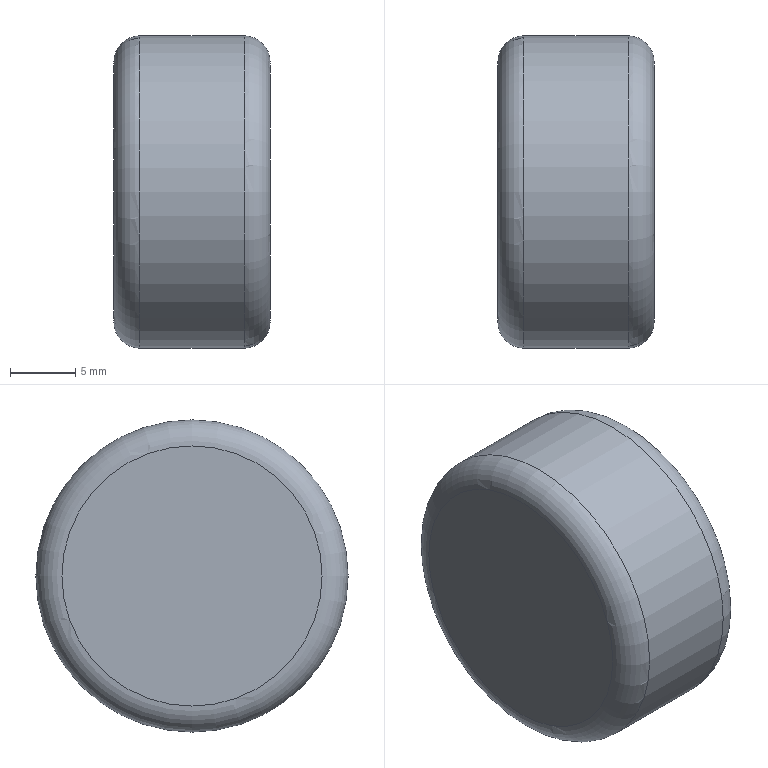Part | NX | features solid 2 | 1 solid | 5 faces | box 12 x 24 x 24 mm | volume 5304 mm3 | plane 2 | torus 2 | cylinder 1 | commonest cylinder face diameters 24 x1
STEP:
#1=CARTESIAN_POINT('',(-73.,145.3,106.));
#2=VERTEX_POINT('',#1);
#3=CARTESIAN_POINT('',(-73.,145.3,96.));
#4=DIRECTION('',(-1.,0.,0.));
#5=DIRECTION('',(0.,0.,1.));
#6=AXIS2_PLACEMENT_3D('',#3,#4,#5);
#7=CIRCLE('',#6,10.);
#8=EDGE_CURVE('',#2,#2,#7,.T.);
#9=ORIENTED_EDGE('',*,*,#8,.T.);
#10=EDGE_LOOP('',(#9));
#11=FACE_BOUND('',#10,.T.);
#12=CARTESIAN_POINT('',(-73.,145.3,96.));
#13=DIRECTION('',(-1.,0.,0.));
#14=DIRECTION('',(0.,0.,1.));
#15=AXIS2_PLACEMENT_3D('',#12,#13,#14);
#16=PLANE('',#15);
#17=ADVANCED_FACE('',(#11),#16,.T.);
#18=CARTESIAN_POINT('',(-61.,145.3,86.));
#19=VERTEX_POINT('',#18);
#20=CARTESIAN_POINT('',(-61.,145.3,96.));
#21=DIRECTION('',(1.,0.,0.));
#22=DIRECTION('',(0.,0.,-1.));
#23=AXIS2_PLACEMENT_3D('',#20,#21,#22);
#24=CIRCLE('',#23,10.);
#25=EDGE_CURVE('',#19,#19,#24,.T.);
#26=ORIENTED_EDGE('',*,*,#25,.T.);
#27=EDGE_LOOP('',(#26));
#28=FACE_BOUND('',#27,.T.);
#29=CARTESIAN_POINT('',(-61.,145.3,96.));
#30=DIRECTION('',(1.,0.,0.));
#31=DIRECTION('',(0.,0.,-1.));
#32=AXIS2_PLACEMENT_3D('',#29,#30,#31);
#33=PLANE('',#32);
#34=ADVANCED_FACE('',(#28),#33,.T.);
#35=CARTESIAN_POINT('',(-71.,145.3,108.));
#36=VERTEX_POINT('',#35);
#37=CARTESIAN_POINT('',(-71.,145.3,96.));
#38=DIRECTION('',(-1.,0.,0.));
#39=DIRECTION('',(0.,0.,1.));
#40=AXIS2_PLACEMENT_3D('',#37,#38,#39);
#41=CIRCLE('',#40,12.);
#42=EDGE_CURVE('',#36,#36,#41,.F.);
#43=ORIENTED_EDGE('',*,*,#42,.T.);
#44=EDGE_LOOP('',(#43));
#45=FACE_BOUND('',#44,.T.);
#46=CARTESIAN_POINT('',(-63.,145.3,84.));
#47=VERTEX_POINT('',#46);
#48=CARTESIAN_POINT('',(-63.,145.3,96.));
#49=DIRECTION('',(1.,0.,0.));
#50=DIRECTION('',(0.,0.,-1.));
#51=AXIS2_PLACEMENT_3D('',#48,#49,#50);
#52=CIRCLE('',#51,12.);
#53=EDGE_CURVE('',#47,#47,#52,.F.);
#54=ORIENTED_EDGE('',*,*,#53,.T.);
#55=EDGE_LOOP('',(#54));
#56=FACE_BOUND('',#55,.T.);
#57=CARTESIAN_POINT('',(-61.,145.3,96.));
#58=DIRECTION('',(-1.,0.,0.));
#59=DIRECTION('',(0.,0.,1.));
#60=AXIS2_PLACEMENT_3D('',#57,#58,#59);
#61=CYLINDRICAL_SURFACE('',#60,12.);
#62=ADVANCED_FACE('',(#45,#56),#61,.T.);
#63=ORIENTED_EDGE('',*,*,#8,.F.);
#64=EDGE_LOOP('',(#63));
#65=FACE_BOUND('',#64,.T.);
#66=ORIENTED_EDGE('',*,*,#42,.F.);
#67=EDGE_LOOP('',(#66));
#68=FACE_BOUND('',#67,.T.);
#69=CARTESIAN_POINT('',(-71.,145.3,96.));
#70=DIRECTION('',(-1.,0.,0.));
#71=DIRECTION('',(0.,0.,1.));
#72=AXIS2_PLACEMENT_3D('',#69,#70,#71);
#73=TOROIDAL_SURFACE('',#72,10.,2.);
#74=ADVANCED_FACE('',(#65,#68),#73,.T.);
#75=ORIENTED_EDGE('',*,*,#25,.F.);
#76=EDGE_LOOP('',(#75));
#77=FACE_BOUND('',#76,.T.);
#78=ORIENTED_EDGE('',*,*,#53,.F.);
#79=EDGE_LOOP('',(#78));
#80=FACE_BOUND('',#79,.T.);
#81=CARTESIAN_POINT('',(-63.,145.3,96.));
#82=DIRECTION('',(1.,0.,0.));
#83=DIRECTION('',(0.,0.,-1.));
#84=AXIS2_PLACEMENT_3D('',#81,#82,#83);
#85=TOROIDAL_SURFACE('',#84,10.,2.);
#86=ADVANCED_FACE('',(#77,#80),#85,.T.);
#87=CLOSED_SHELL('',(#17,#34,#62,#74,#86));
#88=MANIFOLD_SOLID_BREP('',#87);
#89=(LENGTH_UNIT()NAMED_UNIT(*)SI_UNIT(.MILLI.,.METRE.));
#90=UNCERTAINTY_MEASURE_WITH_UNIT(LENGTH_MEASURE(0.00001),#89,'','');
#91=(NAMED_UNIT(*)PLANE_ANGLE_UNIT()SI_UNIT($,.RADIAN.));
#92=(NAMED_UNIT(*)SI_UNIT($,.STERADIAN.)SOLID_ANGLE_UNIT());
#93=(GEOMETRIC_REPRESENTATION_CONTEXT(3)GLOBAL_UNCERTAINTY_ASSIGNED_CONTEXT((#90))GLOBAL_UNIT_ASSIGNED_CONTEXT((#89,#91,#92))REPRESENTATION_CONTEXT('',''));
#94=ADVANCED_BREP_SHAPE_REPRESENTATION('',(#88),#93);